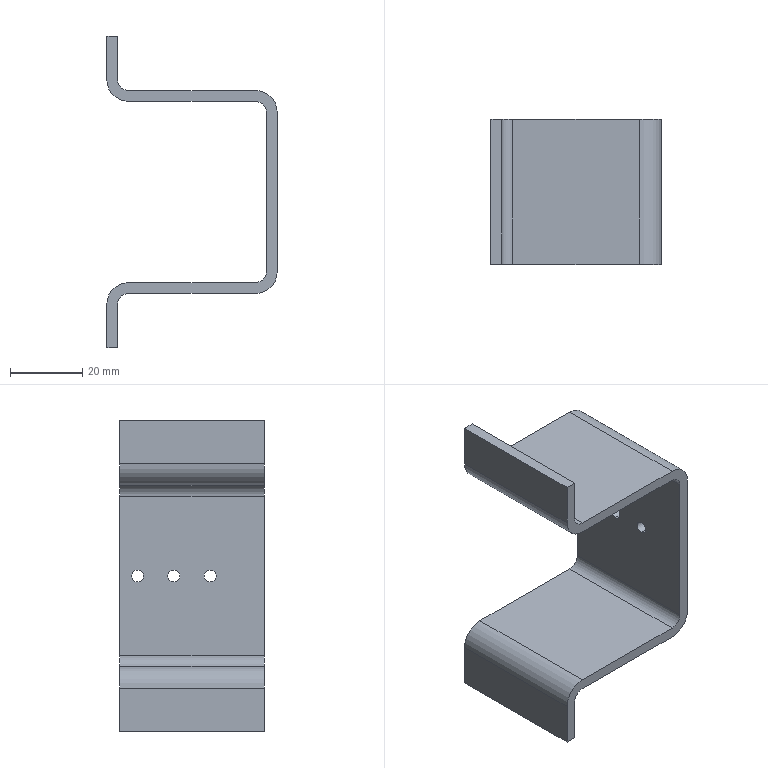Part | SolidWorks | features Fillet 2, Extrusion 1, HoleWzd 1, MoveFace 1 | 1 solid | 28 faces | box 47 x 40 x 86 mm | volume 19876 mm3 | cylinder 14 | plane 14 | commonest cylinder face diameters 3.3 x6 6 x4 12 x4
STEP:
#1=CARTESIAN_POINT('',(-1.5,35.,1.65));
#2=VERTEX_POINT('',#1);
#3=CARTESIAN_POINT('',(-1.5,35.,-1.65));
#4=VERTEX_POINT('',#3);
#5=CARTESIAN_POINT('',(-1.5,35.,0.));
#6=DIRECTION('',(1.,0.,0.));
#7=DIRECTION('',(0.,0.,-1.));
#8=AXIS2_PLACEMENT_3D('',#5,#6,#7);
#9=CIRCLE('',#8,1.65);
#10=EDGE_CURVE('',#2,#4,#9,.T.);
#11=ORIENTED_EDGE('',*,*,#10,.F.);
#12=CARTESIAN_POINT('',(1.5,35.,1.65));
#13=VERTEX_POINT('',#12);
#14=CARTESIAN_POINT('',(1.5,35.,1.65));
#15=DIRECTION('',(1.,0.,0.));
#16=VECTOR('',#15,1000.);
#17=LINE('',#14,#16);
#18=EDGE_CURVE('',#2,#13,#17,.T.);
#19=ORIENTED_EDGE('',*,*,#18,.T.);
#20=CARTESIAN_POINT('',(1.5,35.,-1.65));
#21=VERTEX_POINT('',#20);
#22=CARTESIAN_POINT('',(1.5,35.,0.));
#23=DIRECTION('',(1.,0.,0.));
#24=DIRECTION('',(0.,0.,-1.));
#25=AXIS2_PLACEMENT_3D('',#22,#23,#24);
#26=CIRCLE('',#25,1.65);
#27=EDGE_CURVE('',#13,#21,#26,.T.);
#28=ORIENTED_EDGE('',*,*,#27,.T.);
#29=CARTESIAN_POINT('',(1.5,35.,-1.65));
#30=DIRECTION('',(1.,0.,0.));
#31=VECTOR('',#30,1000.);
#32=LINE('',#29,#31);
#33=EDGE_CURVE('',#4,#21,#32,.T.);
#34=ORIENTED_EDGE('',*,*,#33,.F.);
#35=EDGE_LOOP('',(#11,#19,#28,#34));
#36=FACE_OUTER_BOUND('',#35,.T.);
#37=CARTESIAN_POINT('',(1.5,35.,0.));
#38=DIRECTION('',(1.,0.,0.));
#39=DIRECTION('',(0.,0.,-1.));
#40=AXIS2_PLACEMENT_3D('',#37,#38,#39);
#41=CYLINDRICAL_SURFACE('',#40,1.65);
#42=ADVANCED_FACE('',(#36),#41,.F.);
#43=CARTESIAN_POINT('',(-1.5,25.,1.65));
#44=VERTEX_POINT('',#43);
#45=CARTESIAN_POINT('',(-1.5,25.,-1.65));
#46=VERTEX_POINT('',#45);
#47=CARTESIAN_POINT('',(-1.5,25.,0.));
#48=DIRECTION('',(1.,0.,0.));
#49=DIRECTION('',(0.,0.,-1.));
#50=AXIS2_PLACEMENT_3D('',#47,#48,#49);
#51=CIRCLE('',#50,1.65);
#52=EDGE_CURVE('',#44,#46,#51,.T.);
#53=ORIENTED_EDGE('',*,*,#52,.F.);
#54=CARTESIAN_POINT('',(1.5,25.,1.65));
#55=VERTEX_POINT('',#54);
#56=CARTESIAN_POINT('',(1.5,25.,1.65));
#57=DIRECTION('',(1.,0.,0.));
#58=VECTOR('',#57,1000.);
#59=LINE('',#56,#58);
#60=EDGE_CURVE('',#44,#55,#59,.T.);
#61=ORIENTED_EDGE('',*,*,#60,.T.);
#62=CARTESIAN_POINT('',(1.5,25.,-1.65));
#63=VERTEX_POINT('',#62);
#64=CARTESIAN_POINT('',(1.5,25.,0.));
#65=DIRECTION('',(1.,0.,0.));
#66=DIRECTION('',(0.,0.,-1.));
#67=AXIS2_PLACEMENT_3D('',#64,#65,#66);
#68=CIRCLE('',#67,1.65);
#69=EDGE_CURVE('',#55,#63,#68,.T.);
#70=ORIENTED_EDGE('',*,*,#69,.T.);
#71=CARTESIAN_POINT('',(1.5,25.,-1.65));
#72=DIRECTION('',(1.,0.,0.));
#73=VECTOR('',#72,1000.);
#74=LINE('',#71,#73);
#75=EDGE_CURVE('',#46,#63,#74,.T.);
#76=ORIENTED_EDGE('',*,*,#75,.F.);
#77=EDGE_LOOP('',(#53,#61,#70,#76));
#78=FACE_OUTER_BOUND('',#77,.T.);
#79=CARTESIAN_POINT('',(1.5,25.,0.));
#80=DIRECTION('',(1.,0.,0.));
#81=DIRECTION('',(0.,0.,-1.));
#82=AXIS2_PLACEMENT_3D('',#79,#80,#81);
#83=CYLINDRICAL_SURFACE('',#82,1.65);
#84=ADVANCED_FACE('',(#78),#83,.F.);
#85=CARTESIAN_POINT('',(-1.5,15.,1.65));
#86=VERTEX_POINT('',#85);
#87=CARTESIAN_POINT('',(-1.5,15.,-1.65));
#88=VERTEX_POINT('',#87);
#89=CARTESIAN_POINT('',(-1.5,15.,0.));
#90=DIRECTION('',(1.,0.,0.));
#91=DIRECTION('',(0.,0.,-1.));
#92=AXIS2_PLACEMENT_3D('',#89,#90,#91);
#93=CIRCLE('',#92,1.65);
#94=EDGE_CURVE('',#86,#88,#93,.T.);
#95=ORIENTED_EDGE('',*,*,#94,.F.);
#96=CARTESIAN_POINT('',(1.5,15.,1.65));
#97=VERTEX_POINT('',#96);
#98=CARTESIAN_POINT('',(1.5,15.,1.65));
#99=DIRECTION('',(1.,0.,0.));
#100=VECTOR('',#99,1000.);
#101=LINE('',#98,#100);
#102=EDGE_CURVE('',#86,#97,#101,.T.);
#103=ORIENTED_EDGE('',*,*,#102,.T.);
#104=CARTESIAN_POINT('',(1.5,15.,-1.65));
#105=VERTEX_POINT('',#104);
#106=CARTESIAN_POINT('',(1.5,15.,0.));
#107=DIRECTION('',(1.,0.,0.));
#108=DIRECTION('',(0.,0.,-1.));
#109=AXIS2_PLACEMENT_3D('',#106,#107,#108);
#110=CIRCLE('',#109,1.65);
#111=EDGE_CURVE('',#97,#105,#110,.T.);
#112=ORIENTED_EDGE('',*,*,#111,.T.);
#113=CARTESIAN_POINT('',(1.5,15.,-1.65));
#114=DIRECTION('',(1.,0.,0.));
#115=VECTOR('',#114,1000.);
#116=LINE('',#113,#115);
#117=EDGE_CURVE('',#88,#105,#116,.T.);
#118=ORIENTED_EDGE('',*,*,#117,.F.);
#119=EDGE_LOOP('',(#95,#103,#112,#118));
#120=FACE_OUTER_BOUND('',#119,.T.);
#121=CARTESIAN_POINT('',(1.5,15.,0.));
#122=DIRECTION('',(1.,0.,0.));
#123=DIRECTION('',(0.,0.,-1.));
#124=AXIS2_PLACEMENT_3D('',#121,#122,#123);
#125=CYLINDRICAL_SURFACE('',#124,1.65);
#126=ADVANCED_FACE('',(#120),#125,.F.);
#127=CARTESIAN_POINT('',(-4.5,40.,-28.));
#128=VERTEX_POINT('',#127);
#129=CARTESIAN_POINT('',(-39.5,40.,-28.));
#130=VERTEX_POINT('',#129);
#131=CARTESIAN_POINT('',(1.5,40.,-28.));
#132=DIRECTION('',(-1.,0.,0.));
#133=VECTOR('',#132,1000.);
#134=LINE('',#131,#133);
#135=EDGE_CURVE('',#128,#130,#134,.T.);
#136=ORIENTED_EDGE('',*,*,#135,.F.);
#137=CARTESIAN_POINT('',(-4.5,0.,-28.));
#138=VERTEX_POINT('',#137);
#139=CARTESIAN_POINT('',(-4.5,40.,-28.));
#140=DIRECTION('',(0.,-1.,0.));
#141=VECTOR('',#140,1000.);
#142=LINE('',#139,#141);
#143=EDGE_CURVE('',#128,#138,#142,.T.);
#144=ORIENTED_EDGE('',*,*,#143,.T.);
#145=CARTESIAN_POINT('',(-39.5,0.,-28.));
#146=VERTEX_POINT('',#145);
#147=CARTESIAN_POINT('',(1.5,0.,-28.));
#148=DIRECTION('',(-1.,0.,0.));
#149=VECTOR('',#148,1000.);
#150=LINE('',#147,#149);
#151=EDGE_CURVE('',#138,#146,#150,.T.);
#152=ORIENTED_EDGE('',*,*,#151,.T.);
#153=CARTESIAN_POINT('',(-39.5,40.,-28.));
#154=DIRECTION('',(0.,1.,0.));
#155=VECTOR('',#154,1000.);
#156=LINE('',#153,#155);
#157=EDGE_CURVE('',#146,#130,#156,.T.);
#158=ORIENTED_EDGE('',*,*,#157,.T.);
#159=EDGE_LOOP('',(#136,#144,#152,#158));
#160=FACE_OUTER_BOUND('',#159,.T.);
#161=CARTESIAN_POINT('',(1.5,40.,-28.));
#162=DIRECTION('',(0.,0.,1.));
#163=DIRECTION('',(1.,0.,0.));
#164=AXIS2_PLACEMENT_3D('',#161,#162,#163);
#165=PLANE('',#164);
#166=ADVANCED_FACE('',(#160),#165,.F.);
#167=CARTESIAN_POINT('',(-42.5,40.,-31.));
#168=VERTEX_POINT('',#167);
#169=CARTESIAN_POINT('',(-42.5,40.,-43.));
#170=VERTEX_POINT('',#169);
#171=CARTESIAN_POINT('',(-42.5,40.,-28.));
#172=DIRECTION('',(0.,0.,-1.));
#173=VECTOR('',#172,1000.);
#174=LINE('',#171,#173);
#175=EDGE_CURVE('',#168,#170,#174,.T.);
#176=ORIENTED_EDGE('',*,*,#175,.F.);
#177=CARTESIAN_POINT('',(-42.5,0.,-31.));
#178=VERTEX_POINT('',#177);
#179=CARTESIAN_POINT('',(-42.5,0.,-31.));
#180=DIRECTION('',(0.,-1.,0.));
#181=VECTOR('',#180,1000.);
#182=LINE('',#179,#181);
#183=EDGE_CURVE('',#168,#178,#182,.T.);
#184=ORIENTED_EDGE('',*,*,#183,.T.);
#185=CARTESIAN_POINT('',(-42.5,0.,-43.));
#186=VERTEX_POINT('',#185);
#187=CARTESIAN_POINT('',(-42.5,0.,-28.));
#188=DIRECTION('',(0.,0.,-1.));
#189=VECTOR('',#188,1000.);
#190=LINE('',#187,#189);
#191=EDGE_CURVE('',#178,#186,#190,.T.);
#192=ORIENTED_EDGE('',*,*,#191,.T.);
#193=CARTESIAN_POINT('',(-42.5,40.,-43.));
#194=DIRECTION('',(0.,-1.,0.));
#195=VECTOR('',#194,1000.);
#196=LINE('',#193,#195);
#197=EDGE_CURVE('',#170,#186,#196,.T.);
#198=ORIENTED_EDGE('',*,*,#197,.F.);
#199=EDGE_LOOP('',(#176,#184,#192,#198));
#200=FACE_OUTER_BOUND('',#199,.T.);
#201=CARTESIAN_POINT('',(-42.5,40.,-28.));
#202=DIRECTION('',(-1.,0.,0.));
#203=DIRECTION('',(0.,0.,1.));
#204=AXIS2_PLACEMENT_3D('',#201,#202,#203);
#205=PLANE('',#204);
#206=ADVANCED_FACE('',(#200),#205,.F.);
#207=CARTESIAN_POINT('',(-45.5,0.,-43.));
#208=VERTEX_POINT('',#207);
#209=CARTESIAN_POINT('',(-30.5,0.,-43.));
#210=DIRECTION('',(-1.,0.,0.));
#211=VECTOR('',#210,1000.);
#212=LINE('',#209,#211);
#213=EDGE_CURVE('',#186,#208,#212,.T.);
#214=ORIENTED_EDGE('',*,*,#213,.T.);
#215=CARTESIAN_POINT('',(-45.5,40.,-43.));
#216=VERTEX_POINT('',#215);
#217=CARTESIAN_POINT('',(-45.5,40.,-43.));
#218=DIRECTION('',(0.,-1.,0.));
#219=VECTOR('',#218,1000.);
#220=LINE('',#217,#219);
#221=EDGE_CURVE('',#216,#208,#220,.T.);
#222=ORIENTED_EDGE('',*,*,#221,.F.);
#223=CARTESIAN_POINT('',(-30.5,40.,-43.));
#224=DIRECTION('',(-1.,0.,0.));
#225=VECTOR('',#224,1000.);
#226=LINE('',#223,#225);
#227=EDGE_CURVE('',#170,#216,#226,.T.);
#228=ORIENTED_EDGE('',*,*,#227,.F.);
#229=ORIENTED_EDGE('',*,*,#197,.T.);
#230=EDGE_LOOP('',(#214,#222,#228,#229));
#231=FACE_OUTER_BOUND('',#230,.T.);
#232=CARTESIAN_POINT('',(-30.5,40.,-43.));
#233=DIRECTION('',(0.,0.,1.));
#234=DIRECTION('',(1.,0.,0.));
#235=AXIS2_PLACEMENT_3D('',#232,#233,#234);
#236=PLANE('',#235);
#237=ADVANCED_FACE('',(#231),#236,.F.);
#238=CARTESIAN_POINT('',(-45.5,0.,-31.));
#239=VERTEX_POINT('',#238);
#240=CARTESIAN_POINT('',(-45.5,0.,-25.));
#241=DIRECTION('',(0.,0.,1.));
#242=VECTOR('',#241,1000.);
#243=LINE('',#240,#242);
#244=EDGE_CURVE('',#208,#239,#243,.T.);
#245=ORIENTED_EDGE('',*,*,#244,.T.);
#246=CARTESIAN_POINT('',(-45.5,40.,-31.));
#247=VERTEX_POINT('',#246);
#248=CARTESIAN_POINT('',(-45.5,40.,-31.));
#249=DIRECTION('',(0.,1.,0.));
#250=VECTOR('',#249,1000.);
#251=LINE('',#248,#250);
#252=EDGE_CURVE('',#239,#247,#251,.T.);
#253=ORIENTED_EDGE('',*,*,#252,.T.);
#254=CARTESIAN_POINT('',(-45.5,40.,-28.));
#255=DIRECTION('',(0.,0.,1.));
#256=VECTOR('',#255,1000.);
#257=LINE('',#254,#256);
#258=EDGE_CURVE('',#216,#247,#257,.T.);
#259=ORIENTED_EDGE('',*,*,#258,.F.);
#260=ORIENTED_EDGE('',*,*,#221,.T.);
#261=EDGE_LOOP('',(#245,#253,#259,#260));
#262=FACE_OUTER_BOUND('',#261,.T.);
#263=CARTESIAN_POINT('',(-45.5,40.,-25.));
#264=DIRECTION('',(1.,0.,0.));
#265=DIRECTION('',(0.,0.,-1.));
#266=AXIS2_PLACEMENT_3D('',#263,#264,#265);
#267=PLANE('',#266);
#268=ADVANCED_FACE('',(#262),#267,.F.);
#269=CARTESIAN_POINT('',(-39.5,40.,-25.));
#270=VERTEX_POINT('',#269);
#271=CARTESIAN_POINT('',(-4.5,40.,-25.));
#272=VERTEX_POINT('',#271);
#273=CARTESIAN_POINT('',(-1.5,40.,-25.));
#274=DIRECTION('',(1.,0.,0.));
#275=VECTOR('',#274,1000.);
#276=LINE('',#273,#275);
#277=EDGE_CURVE('',#270,#272,#276,.T.);
#278=ORIENTED_EDGE('',*,*,#277,.F.);
#279=CARTESIAN_POINT('',(-39.5,0.,-25.));
#280=VERTEX_POINT('',#279);
#281=CARTESIAN_POINT('',(-39.5,40.,-25.));
#282=DIRECTION('',(0.,-1.,0.));
#283=VECTOR('',#282,1000.);
#284=LINE('',#281,#283);
#285=EDGE_CURVE('',#270,#280,#284,.T.);
#286=ORIENTED_EDGE('',*,*,#285,.T.);
#287=CARTESIAN_POINT('',(-4.5,0.,-25.));
#288=VERTEX_POINT('',#287);
#289=CARTESIAN_POINT('',(-1.5,0.,-25.));
#290=DIRECTION('',(1.,0.,0.));
#291=VECTOR('',#290,1000.);
#292=LINE('',#289,#291);
#293=EDGE_CURVE('',#280,#288,#292,.T.);
#294=ORIENTED_EDGE('',*,*,#293,.T.);
#295=CARTESIAN_POINT('',(-4.5,40.,-25.));
#296=DIRECTION('',(0.,1.,0.));
#297=VECTOR('',#296,1000.);
#298=LINE('',#295,#297);
#299=EDGE_CURVE('',#288,#272,#298,.T.);
#300=ORIENTED_EDGE('',*,*,#299,.T.);
#301=EDGE_LOOP('',(#278,#286,#294,#300));
#302=FACE_OUTER_BOUND('',#301,.T.);
#303=CARTESIAN_POINT('',(-1.5,40.,-25.));
#304=DIRECTION('',(0.,0.,-1.));
#305=DIRECTION('',(-1.,0.,0.));
#306=AXIS2_PLACEMENT_3D('',#303,#304,#305);
#307=PLANE('',#306);
#308=ADVANCED_FACE('',(#302),#307,.F.);
#309=CARTESIAN_POINT('',(-1.5,35.,0.));
#310=DIRECTION('',(1.,0.,0.));
#311=DIRECTION('',(0.,0.,-1.));
#312=AXIS2_PLACEMENT_3D('',#309,#310,#311);
#313=CIRCLE('',#312,1.65);
#314=EDGE_CURVE('',#4,#2,#313,.T.);
#315=ORIENTED_EDGE('',*,*,#314,.T.);
#316=ORIENTED_EDGE('',*,*,#10,.T.);
#317=EDGE_LOOP('',(#315,#316));
#318=FACE_BOUND('',#317,.T.);
#319=CARTESIAN_POINT('',(-1.5,25.,0.));
#320=DIRECTION('',(1.,0.,0.));
#321=DIRECTION('',(0.,0.,-1.));
#322=AXIS2_PLACEMENT_3D('',#319,#320,#321);
#323=CIRCLE('',#322,1.65);
#324=EDGE_CURVE('',#46,#44,#323,.T.);
#325=ORIENTED_EDGE('',*,*,#324,.T.);
#326=ORIENTED_EDGE('',*,*,#52,.T.);
#327=EDGE_LOOP('',(#325,#326));
#328=FACE_BOUND('',#327,.T.);
#329=CARTESIAN_POINT('',(-1.5,15.,0.));
#330=DIRECTION('',(1.,0.,0.));
#331=DIRECTION('',(0.,0.,-1.));
#332=AXIS2_PLACEMENT_3D('',#329,#330,#331);
#333=CIRCLE('',#332,1.65);
#334=EDGE_CURVE('',#88,#86,#333,.T.);
#335=ORIENTED_EDGE('',*,*,#334,.T.);
#336=ORIENTED_EDGE('',*,*,#94,.T.);
#337=EDGE_LOOP('',(#335,#336));
#338=FACE_BOUND('',#337,.T.);
#339=CARTESIAN_POINT('',(-1.5,0.,-22.));
#340=VERTEX_POINT('',#339);
#341=CARTESIAN_POINT('',(-1.5,0.,22.));
#342=VERTEX_POINT('',#341);
#343=CARTESIAN_POINT('',(-1.5,0.,25.));
#344=DIRECTION('',(0.,0.,1.));
#345=VECTOR('',#344,1000.);
#346=LINE('',#343,#345);
#347=EDGE_CURVE('',#340,#342,#346,.T.);
#348=ORIENTED_EDGE('',*,*,#347,.T.);
#349=CARTESIAN_POINT('',(-1.5,40.,22.));
#350=VERTEX_POINT('',#349);
#351=CARTESIAN_POINT('',(-1.5,40.,22.));
#352=DIRECTION('',(0.,1.,0.));
#353=VECTOR('',#352,1000.);
#354=LINE('',#351,#353);
#355=EDGE_CURVE('',#342,#350,#354,.T.);
#356=ORIENTED_EDGE('',*,*,#355,.T.);
#357=CARTESIAN_POINT('',(-1.5,40.,-22.));
#358=VERTEX_POINT('',#357);
#359=CARTESIAN_POINT('',(-1.5,40.,25.));
#360=DIRECTION('',(0.,0.,1.));
#361=VECTOR('',#360,1000.);
#362=LINE('',#359,#361);
#363=EDGE_CURVE('',#358,#350,#362,.T.);
#364=ORIENTED_EDGE('',*,*,#363,.F.);
#365=CARTESIAN_POINT('',(-1.5,0.,-22.));
#366=DIRECTION('',(0.,-1.,0.));
#367=VECTOR('',#366,1000.);
#368=LINE('',#365,#367);
#369=EDGE_CURVE('',#358,#340,#368,.T.);
#370=ORIENTED_EDGE('',*,*,#369,.T.);
#371=EDGE_LOOP('',(#348,#356,#364,#370));
#372=FACE_OUTER_BOUND('',#371,.T.);
#373=CARTESIAN_POINT('',(-1.5,40.,25.));
#374=DIRECTION('',(1.,0.,0.));
#375=DIRECTION('',(0.,0.,-1.));
#376=AXIS2_PLACEMENT_3D('',#373,#374,#375);
#377=PLANE('',#376);
#378=ADVANCED_FACE('',(#318,#328,#338,#372),#377,.F.);
#379=CARTESIAN_POINT('',(-4.5,0.,25.));
#380=VERTEX_POINT('',#379);
#381=CARTESIAN_POINT('',(-39.5,0.,25.));
#382=VERTEX_POINT('',#381);
#383=CARTESIAN_POINT('',(-1.5,0.,25.));
#384=DIRECTION('',(-1.,0.,0.));
#385=VECTOR('',#384,1000.);
#386=LINE('',#383,#385);
#387=EDGE_CURVE('',#380,#382,#386,.T.);
#388=ORIENTED_EDGE('',*,*,#387,.T.);
#389=CARTESIAN_POINT('',(-39.5,40.,25.));
#390=VERTEX_POINT('',#389);
#391=CARTESIAN_POINT('',(-39.5,40.,25.));
#392=DIRECTION('',(0.,1.,0.));
#393=VECTOR('',#392,1000.);
#394=LINE('',#391,#393);
#395=EDGE_CURVE('',#382,#390,#394,.T.);
#396=ORIENTED_EDGE('',*,*,#395,.T.);
#397=CARTESIAN_POINT('',(-4.5,40.,25.));
#398=VERTEX_POINT('',#397);
#399=CARTESIAN_POINT('',(-1.5,40.,25.));
#400=DIRECTION('',(-1.,0.,0.));
#401=VECTOR('',#400,1000.);
#402=LINE('',#399,#401);
#403=EDGE_CURVE('',#398,#390,#402,.T.);
#404=ORIENTED_EDGE('',*,*,#403,.F.);
#405=CARTESIAN_POINT('',(-4.5,0.,25.));
#406=DIRECTION('',(0.,-1.,0.));
#407=VECTOR('',#406,1000.);
#408=LINE('',#405,#407);
#409=EDGE_CURVE('',#398,#380,#408,.T.);
#410=ORIENTED_EDGE('',*,*,#409,.T.);
#411=EDGE_LOOP('',(#388,#396,#404,#410));
#412=FACE_OUTER_BOUND('',#411,.T.);
#413=CARTESIAN_POINT('',(-1.5,40.,25.));
#414=DIRECTION('',(0.,0.,1.));
#415=DIRECTION('',(1.,0.,0.));
#416=AXIS2_PLACEMENT_3D('',#413,#414,#415);
#417=PLANE('',#416);
#418=ADVANCED_FACE('',(#412),#417,.F.);
#419=CARTESIAN_POINT('',(-45.5,40.,31.));
#420=VERTEX_POINT('',#419);
#421=CARTESIAN_POINT('',(-45.5,40.,43.));
#422=VERTEX_POINT('',#421);
#423=CARTESIAN_POINT('',(-45.5,40.,25.));
#424=DIRECTION('',(0.,0.,1.));
#425=VECTOR('',#424,1000.);
#426=LINE('',#423,#425);
#427=EDGE_CURVE('',#420,#422,#426,.T.);
#428=ORIENTED_EDGE('',*,*,#427,.F.);
#429=CARTESIAN_POINT('',(-45.5,0.,31.));
#430=VERTEX_POINT('',#429);
#431=CARTESIAN_POINT('',(-45.5,40.,31.));
#432=DIRECTION('',(0.,-1.,0.));
#433=VECTOR('',#432,1000.);
#434=LINE('',#431,#433);
#435=EDGE_CURVE('',#420,#430,#434,.T.);
#436=ORIENTED_EDGE('',*,*,#435,.T.);
#437=CARTESIAN_POINT('',(-45.5,0.,43.));
#438=VERTEX_POINT('',#437);
#439=CARTESIAN_POINT('',(-45.5,0.,28.));
#440=DIRECTION('',(0.,0.,1.));
#441=VECTOR('',#440,1000.);
#442=LINE('',#439,#441);
#443=EDGE_CURVE('',#430,#438,#442,.T.);
#444=ORIENTED_EDGE('',*,*,#443,.T.);
#445=CARTESIAN_POINT('',(-45.5,40.,43.));
#446=DIRECTION('',(0.,-1.,0.));
#447=VECTOR('',#446,1000.);
#448=LINE('',#445,#447);
#449=EDGE_CURVE('',#422,#438,#448,.T.);
#450=ORIENTED_EDGE('',*,*,#449,.F.);
#451=EDGE_LOOP('',(#428,#436,#444,#450));
#452=FACE_OUTER_BOUND('',#451,.T.);
#453=CARTESIAN_POINT('',(-45.5,40.,28.));
#454=DIRECTION('',(1.,0.,0.));
#455=DIRECTION('',(0.,0.,-1.));
#456=AXIS2_PLACEMENT_3D('',#453,#454,#455);
#457=PLANE('',#456);
#458=ADVANCED_FACE('',(#452),#457,.F.);
#459=CARTESIAN_POINT('',(-42.5,0.,43.));
#460=VERTEX_POINT('',#459);
#461=CARTESIAN_POINT('',(-30.5,0.,43.));
#462=DIRECTION('',(1.,0.,0.));
#463=VECTOR('',#462,1000.);
#464=LINE('',#461,#463);
#465=EDGE_CURVE('',#438,#460,#464,.T.);
#466=ORIENTED_EDGE('',*,*,#465,.T.);
#467=CARTESIAN_POINT('',(-42.5,40.,43.));
#468=VERTEX_POINT('',#467);
#469=CARTESIAN_POINT('',(-42.5,40.,43.));
#470=DIRECTION('',(0.,-1.,0.));
#471=VECTOR('',#470,1000.);
#472=LINE('',#469,#471);
#473=EDGE_CURVE('',#468,#460,#472,.T.);
#474=ORIENTED_EDGE('',*,*,#473,.F.);
#475=CARTESIAN_POINT('',(-30.5,40.,43.));
#476=DIRECTION('',(1.,0.,0.));
#477=VECTOR('',#476,1000.);
#478=LINE('',#475,#477);
#479=EDGE_CURVE('',#422,#468,#478,.T.);
#480=ORIENTED_EDGE('',*,*,#479,.F.);
#481=ORIENTED_EDGE('',*,*,#449,.T.);
#482=EDGE_LOOP('',(#466,#474,#480,#481));
#483=FACE_OUTER_BOUND('',#482,.T.);
#484=CARTESIAN_POINT('',(-30.5,40.,43.));
#485=DIRECTION('',(0.,0.,-1.));
#486=DIRECTION('',(-1.,0.,0.));
#487=AXIS2_PLACEMENT_3D('',#484,#485,#486);
#488=PLANE('',#487);
#489=ADVANCED_FACE('',(#483),#488,.F.);
#490=CARTESIAN_POINT('',(-42.5,0.,31.));
#491=VERTEX_POINT('',#490);
#492=CARTESIAN_POINT('',(-42.5,0.,28.));
#493=DIRECTION('',(0.,0.,-1.));
#494=VECTOR('',#493,1000.);
#495=LINE('',#492,#494);
#496=EDGE_CURVE('',#460,#491,#495,.T.);
#497=ORIENTED_EDGE('',*,*,#496,.T.);
#498=CARTESIAN_POINT('',(-42.5,40.,31.));
#499=VERTEX_POINT('',#498);
#500=CARTESIAN_POINT('',(-42.5,40.,31.));
#501=DIRECTION('',(0.,1.,0.));
#502=VECTOR('',#501,1000.);
#503=LINE('',#500,#502);
#504=EDGE_CURVE('',#491,#499,#503,.T.);
#505=ORIENTED_EDGE('',*,*,#504,.T.);
#506=CARTESIAN_POINT('',(-42.5,40.,28.));
#507=DIRECTION('',(0.,0.,-1.));
#508=VECTOR('',#507,1000.);
#509=LINE('',#506,#508);
#510=EDGE_CURVE('',#468,#499,#509,.T.);
#511=ORIENTED_EDGE('',*,*,#510,.F.);
#512=ORIENTED_EDGE('',*,*,#473,.T.);
#513=EDGE_LOOP('',(#497,#505,#511,#512));
#514=FACE_OUTER_BOUND('',#513,.T.);
#515=CARTESIAN_POINT('',(-42.5,40.,28.));
#516=DIRECTION('',(-1.,0.,0.));
#517=DIRECTION('',(0.,0.,1.));
#518=AXIS2_PLACEMENT_3D('',#515,#516,#517);
#519=PLANE('',#518);
#520=ADVANCED_FACE('',(#514),#519,.F.);
#521=CARTESIAN_POINT('',(-39.5,0.,28.));
#522=VERTEX_POINT('',#521);
#523=CARTESIAN_POINT('',(-4.5,0.,28.));
#524=VERTEX_POINT('',#523);
#525=CARTESIAN_POINT('',(1.5,0.,28.));
#526=DIRECTION('',(1.,0.,0.));
#527=VECTOR('',#526,1000.);
#528=LINE('',#525,#527);
#529=EDGE_CURVE('',#522,#524,#528,.T.);
#530=ORIENTED_EDGE('',*,*,#529,.T.);
#531=CARTESIAN_POINT('',(-4.5,40.,28.));
#532=VERTEX_POINT('',#531);
#533=CARTESIAN_POINT('',(-4.5,40.,28.));
#534=DIRECTION('',(0.,1.,0.));
#535=VECTOR('',#534,1000.);
#536=LINE('',#533,#535);
#537=EDGE_CURVE('',#524,#532,#536,.T.);
#538=ORIENTED_EDGE('',*,*,#537,.T.);
#539=CARTESIAN_POINT('',(-39.5,40.,28.));
#540=VERTEX_POINT('',#539);
#541=CARTESIAN_POINT('',(1.5,40.,28.));
#542=DIRECTION('',(1.,0.,0.));
#543=VECTOR('',#542,1000.);
#544=LINE('',#541,#543);
#545=EDGE_CURVE('',#540,#532,#544,.T.);
#546=ORIENTED_EDGE('',*,*,#545,.F.);
#547=CARTESIAN_POINT('',(-39.5,0.,28.));
#548=DIRECTION('',(0.,-1.,0.));
#549=VECTOR('',#548,1000.);
#550=LINE('',#547,#549);
#551=EDGE_CURVE('',#540,#522,#550,.T.);
#552=ORIENTED_EDGE('',*,*,#551,.T.);
#553=EDGE_LOOP('',(#530,#538,#546,#552));
#554=FACE_OUTER_BOUND('',#553,.T.);
#555=CARTESIAN_POINT('',(1.5,40.,28.));
#556=DIRECTION('',(0.,0.,-1.));
#557=DIRECTION('',(-1.,0.,0.));
#558=AXIS2_PLACEMENT_3D('',#555,#556,#557);
#559=PLANE('',#558);
#560=ADVANCED_FACE('',(#554),#559,.F.);
#561=CARTESIAN_POINT('',(1.5,35.,0.));
#562=DIRECTION('',(1.,0.,0.));
#563=DIRECTION('',(0.,0.,-1.));
#564=AXIS2_PLACEMENT_3D('',#561,#562,#563);
#565=CIRCLE('',#564,1.65);
#566=EDGE_CURVE('',#21,#13,#565,.T.);
#567=ORIENTED_EDGE('',*,*,#566,.F.);
#568=ORIENTED_EDGE('',*,*,#27,.F.);
#569=EDGE_LOOP('',(#567,#568));
#570=FACE_BOUND('',#569,.T.);
#571=CARTESIAN_POINT('',(1.5,25.,0.));
#572=DIRECTION('',(1.,0.,0.));
#573=DIRECTION('',(0.,0.,-1.));
#574=AXIS2_PLACEMENT_3D('',#571,#572,#573);
#575=CIRCLE('',#574,1.65);
#576=EDGE_CURVE('',#63,#55,#575,.T.);
#577=ORIENTED_EDGE('',*,*,#576,.F.);
#578=ORIENTED_EDGE('',*,*,#69,.F.);
#579=EDGE_LOOP('',(#577,#578));
#580=FACE_BOUND('',#579,.T.);
#581=CARTESIAN_POINT('',(1.5,15.,0.));
#582=DIRECTION('',(1.,0.,0.));
#583=DIRECTION('',(0.,0.,-1.));
#584=AXIS2_PLACEMENT_3D('',#581,#582,#583);
#585=CIRCLE('',#584,1.65);
#586=EDGE_CURVE('',#105,#97,#585,.T.);
#587=ORIENTED_EDGE('',*,*,#586,.F.);
#588=ORIENTED_EDGE('',*,*,#111,.F.);
#589=EDGE_LOOP('',(#587,#588));
#590=FACE_BOUND('',#589,.T.);
#591=CARTESIAN_POINT('',(1.5,40.,22.));
#592=VERTEX_POINT('',#591);
#593=CARTESIAN_POINT('',(1.5,40.,-22.));
#594=VERTEX_POINT('',#593);
#595=CARTESIAN_POINT('',(1.5,40.,-25.));
#596=DIRECTION('',(0.,0.,-1.));
#597=VECTOR('',#596,1000.);
#598=LINE('',#595,#597);
#599=EDGE_CURVE('',#592,#594,#598,.T.);
#600=ORIENTED_EDGE('',*,*,#599,.F.);
#601=CARTESIAN_POINT('',(1.5,0.,22.));
#602=VERTEX_POINT('',#601);
#603=CARTESIAN_POINT('',(1.5,40.,22.));
#604=DIRECTION('',(0.,-1.,0.));
#605=VECTOR('',#604,1000.);
#606=LINE('',#603,#605);
#607=EDGE_CURVE('',#592,#602,#606,.T.);
#608=ORIENTED_EDGE('',*,*,#607,.T.);
#609=CARTESIAN_POINT('',(1.5,0.,-22.));
#610=VERTEX_POINT('',#609);
#611=CARTESIAN_POINT('',(1.5,0.,25.));
#612=DIRECTION('',(0.,0.,-1.));
#613=VECTOR('',#612,1000.);
#614=LINE('',#611,#613);
#615=EDGE_CURVE('',#602,#610,#614,.T.);
#616=ORIENTED_EDGE('',*,*,#615,.T.);
#617=CARTESIAN_POINT('',(1.5,40.,-22.));
#618=DIRECTION('',(0.,1.,0.));
#619=VECTOR('',#618,1000.);
#620=LINE('',#617,#619);
#621=EDGE_CURVE('',#610,#594,#620,.T.);
#622=ORIENTED_EDGE('',*,*,#621,.T.);
#623=EDGE_LOOP('',(#600,#608,#616,#622));
#624=FACE_OUTER_BOUND('',#623,.T.);
#625=CARTESIAN_POINT('',(1.5,40.,25.));
#626=DIRECTION('',(-1.,0.,0.));
#627=DIRECTION('',(0.,0.,1.));
#628=AXIS2_PLACEMENT_3D('',#625,#626,#627);
#629=PLANE('',#628);
#630=ADVANCED_FACE('',(#570,#580,#590,#624),#629,.F.);
#631=ORIENTED_EDGE('',*,*,#403,.T.);
#632=CARTESIAN_POINT('',(-39.5,40.,31.));
#633=DIRECTION('',(0.,1.,0.));
#634=DIRECTION('',(0.,0.,1.));
#635=AXIS2_PLACEMENT_3D('',#632,#633,#634);
#636=CIRCLE('',#635,6.);
#637=EDGE_CURVE('',#390,#420,#636,.T.);
#638=ORIENTED_EDGE('',*,*,#637,.T.);
#639=ORIENTED_EDGE('',*,*,#427,.T.);
#640=ORIENTED_EDGE('',*,*,#479,.T.);
#641=ORIENTED_EDGE('',*,*,#510,.T.);
#642=CARTESIAN_POINT('',(-39.5,40.,31.));
#643=DIRECTION('',(0.,-1.,0.));
#644=DIRECTION('',(0.,0.,1.));
#645=AXIS2_PLACEMENT_3D('',#642,#643,#644);
#646=CIRCLE('',#645,3.);
#647=EDGE_CURVE('',#499,#540,#646,.T.);
#648=ORIENTED_EDGE('',*,*,#647,.T.);
#649=ORIENTED_EDGE('',*,*,#545,.T.);
#650=CARTESIAN_POINT('',(-4.5,40.,22.));
#651=DIRECTION('',(0.,1.,0.));
#652=DIRECTION('',(0.,0.,1.));
#653=AXIS2_PLACEMENT_3D('',#650,#651,#652);
#654=CIRCLE('',#653,6.);
#655=EDGE_CURVE('',#532,#592,#654,.T.);
#656=ORIENTED_EDGE('',*,*,#655,.T.);
#657=ORIENTED_EDGE('',*,*,#599,.T.);
#658=CARTESIAN_POINT('',(-4.5,40.,-22.));
#659=DIRECTION('',(0.,1.,0.));
#660=DIRECTION('',(0.,0.,1.));
#661=AXIS2_PLACEMENT_3D('',#658,#659,#660);
#662=CIRCLE('',#661,6.);
#663=EDGE_CURVE('',#594,#128,#662,.T.);
#664=ORIENTED_EDGE('',*,*,#663,.T.);
#665=ORIENTED_EDGE('',*,*,#135,.T.);
#666=CARTESIAN_POINT('',(-39.5,40.,-31.));
#667=DIRECTION('',(0.,-1.,0.));
#668=DIRECTION('',(0.,0.,1.));
#669=AXIS2_PLACEMENT_3D('',#666,#667,#668);
#670=CIRCLE('',#669,3.);
#671=EDGE_CURVE('',#130,#168,#670,.T.);
#672=ORIENTED_EDGE('',*,*,#671,.T.);
#673=ORIENTED_EDGE('',*,*,#175,.T.);
#674=ORIENTED_EDGE('',*,*,#227,.T.);
#675=ORIENTED_EDGE('',*,*,#258,.T.);
#676=CARTESIAN_POINT('',(-39.5,40.,-31.));
#677=DIRECTION('',(0.,1.,0.));
#678=DIRECTION('',(0.,0.,1.));
#679=AXIS2_PLACEMENT_3D('',#676,#677,#678);
#680=CIRCLE('',#679,6.);
#681=EDGE_CURVE('',#247,#270,#680,.T.);
#682=ORIENTED_EDGE('',*,*,#681,.T.);
#683=ORIENTED_EDGE('',*,*,#277,.T.);
#684=CARTESIAN_POINT('',(-4.5,40.,-22.));
#685=DIRECTION('',(0.,-1.,0.));
#686=DIRECTION('',(0.,0.,1.));
#687=AXIS2_PLACEMENT_3D('',#684,#685,#686);
#688=CIRCLE('',#687,3.);
#689=EDGE_CURVE('',#272,#358,#688,.T.);
#690=ORIENTED_EDGE('',*,*,#689,.T.);
#691=ORIENTED_EDGE('',*,*,#363,.T.);
#692=CARTESIAN_POINT('',(-4.5,40.,22.));
#693=DIRECTION('',(0.,-1.,0.));
#694=DIRECTION('',(0.,0.,1.));
#695=AXIS2_PLACEMENT_3D('',#692,#693,#694);
#696=CIRCLE('',#695,3.);
#697=EDGE_CURVE('',#350,#398,#696,.T.);
#698=ORIENTED_EDGE('',*,*,#697,.T.);
#699=EDGE_LOOP('',(#631,#638,#639,#640,#641,#648,#649,#656,#657,#664,#665,#672,#673,#674,#675,#682,#683,#690,#691,#698));
#700=FACE_OUTER_BOUND('',#699,.T.);
#701=CARTESIAN_POINT('',(0.,40.,0.));
#702=DIRECTION('',(0.,1.,0.));
#703=DIRECTION('',(0.,0.,1.));
#704=AXIS2_PLACEMENT_3D('',#701,#702,#703);
#705=PLANE('',#704);
#706=ADVANCED_FACE('',(#700),#705,.T.);
#707=ORIENTED_EDGE('',*,*,#443,.F.);
#708=CARTESIAN_POINT('',(-39.5,0.,31.));
#709=DIRECTION('',(0.,-1.,0.));
#710=DIRECTION('',(0.,0.,1.));
#711=AXIS2_PLACEMENT_3D('',#708,#709,#710);
#712=CIRCLE('',#711,6.);
#713=EDGE_CURVE('',#430,#382,#712,.T.);
#714=ORIENTED_EDGE('',*,*,#713,.T.);
#715=ORIENTED_EDGE('',*,*,#387,.F.);
#716=CARTESIAN_POINT('',(-4.5,0.,22.));
#717=DIRECTION('',(0.,1.,0.));
#718=DIRECTION('',(0.,0.,1.));
#719=AXIS2_PLACEMENT_3D('',#716,#717,#718);
#720=CIRCLE('',#719,3.);
#721=EDGE_CURVE('',#380,#342,#720,.T.);
#722=ORIENTED_EDGE('',*,*,#721,.T.);
#723=ORIENTED_EDGE('',*,*,#347,.F.);
#724=CARTESIAN_POINT('',(-4.5,0.,-22.));
#725=DIRECTION('',(0.,1.,0.));
#726=DIRECTION('',(0.,0.,1.));
#727=AXIS2_PLACEMENT_3D('',#724,#725,#726);
#728=CIRCLE('',#727,3.);
#729=EDGE_CURVE('',#340,#288,#728,.T.);
#730=ORIENTED_EDGE('',*,*,#729,.T.);
#731=ORIENTED_EDGE('',*,*,#293,.F.);
#732=CARTESIAN_POINT('',(-39.5,0.,-31.));
#733=DIRECTION('',(0.,-1.,0.));
#734=DIRECTION('',(0.,0.,1.));
#735=AXIS2_PLACEMENT_3D('',#732,#733,#734);
#736=CIRCLE('',#735,6.);
#737=EDGE_CURVE('',#280,#239,#736,.T.);
#738=ORIENTED_EDGE('',*,*,#737,.T.);
#739=ORIENTED_EDGE('',*,*,#244,.F.);
#740=ORIENTED_EDGE('',*,*,#213,.F.);
#741=ORIENTED_EDGE('',*,*,#191,.F.);
#742=CARTESIAN_POINT('',(-39.5,0.,-31.));
#743=DIRECTION('',(0.,1.,0.));
#744=DIRECTION('',(0.,0.,1.));
#745=AXIS2_PLACEMENT_3D('',#742,#743,#744);
#746=CIRCLE('',#745,3.);
#747=EDGE_CURVE('',#178,#146,#746,.T.);
#748=ORIENTED_EDGE('',*,*,#747,.T.);
#749=ORIENTED_EDGE('',*,*,#151,.F.);
#750=CARTESIAN_POINT('',(-4.5,0.,-22.));
#751=DIRECTION('',(0.,-1.,0.));
#752=DIRECTION('',(0.,0.,1.));
#753=AXIS2_PLACEMENT_3D('',#750,#751,#752);
#754=CIRCLE('',#753,6.);
#755=EDGE_CURVE('',#138,#610,#754,.T.);
#756=ORIENTED_EDGE('',*,*,#755,.T.);
#757=ORIENTED_EDGE('',*,*,#615,.F.);
#758=CARTESIAN_POINT('',(-4.5,0.,22.));
#759=DIRECTION('',(0.,-1.,0.));
#760=DIRECTION('',(0.,0.,1.));
#761=AXIS2_PLACEMENT_3D('',#758,#759,#760);
#762=CIRCLE('',#761,6.);
#763=EDGE_CURVE('',#602,#524,#762,.T.);
#764=ORIENTED_EDGE('',*,*,#763,.T.);
#765=ORIENTED_EDGE('',*,*,#529,.F.);
#766=CARTESIAN_POINT('',(-39.5,0.,31.));
#767=DIRECTION('',(0.,1.,0.));
#768=DIRECTION('',(0.,0.,1.));
#769=AXIS2_PLACEMENT_3D('',#766,#767,#768);
#770=CIRCLE('',#769,3.);
#771=EDGE_CURVE('',#522,#491,#770,.T.);
#772=ORIENTED_EDGE('',*,*,#771,.T.);
#773=ORIENTED_EDGE('',*,*,#496,.F.);
#774=ORIENTED_EDGE('',*,*,#465,.F.);
#775=EDGE_LOOP('',(#707,#714,#715,#722,#723,#730,#731,#738,#739,#740,#741,#748,#749,#756,#757,#764,#765,#772,#773,#774));
#776=FACE_OUTER_BOUND('',#775,.T.);
#777=CARTESIAN_POINT('',(0.,0.,0.));
#778=DIRECTION('',(0.,1.,0.));
#779=DIRECTION('',(0.,0.,1.));
#780=AXIS2_PLACEMENT_3D('',#777,#778,#779);
#781=PLANE('',#780);
#782=ADVANCED_FACE('',(#776),#781,.F.);
#783=ORIENTED_EDGE('',*,*,#647,.F.);
#784=ORIENTED_EDGE('',*,*,#504,.F.);
#785=ORIENTED_EDGE('',*,*,#771,.F.);
#786=ORIENTED_EDGE('',*,*,#551,.F.);
#787=EDGE_LOOP('',(#783,#784,#785,#786));
#788=FACE_OUTER_BOUND('',#787,.T.);
#789=CARTESIAN_POINT('',(-39.5,40.,31.));
#790=DIRECTION('',(0.,1.,0.));
#791=DIRECTION('',(0.,0.,1.));
#792=AXIS2_PLACEMENT_3D('',#789,#790,#791);
#793=CYLINDRICAL_SURFACE('',#792,3.);
#794=ADVANCED_FACE('',(#788),#793,.F.);
#795=ORIENTED_EDGE('',*,*,#697,.F.);
#796=ORIENTED_EDGE('',*,*,#355,.F.);
#797=ORIENTED_EDGE('',*,*,#721,.F.);
#798=ORIENTED_EDGE('',*,*,#409,.F.);
#799=EDGE_LOOP('',(#795,#796,#797,#798));
#800=FACE_OUTER_BOUND('',#799,.T.);
#801=CARTESIAN_POINT('',(-4.5,40.,22.));
#802=DIRECTION('',(0.,1.,0.));
#803=DIRECTION('',(0.,0.,1.));
#804=AXIS2_PLACEMENT_3D('',#801,#802,#803);
#805=CYLINDRICAL_SURFACE('',#804,3.);
#806=ADVANCED_FACE('',(#800),#805,.F.);
#807=ORIENTED_EDGE('',*,*,#689,.F.);
#808=ORIENTED_EDGE('',*,*,#299,.F.);
#809=ORIENTED_EDGE('',*,*,#729,.F.);
#810=ORIENTED_EDGE('',*,*,#369,.F.);
#811=EDGE_LOOP('',(#807,#808,#809,#810));
#812=FACE_OUTER_BOUND('',#811,.T.);
#813=CARTESIAN_POINT('',(-4.5,40.,-22.));
#814=DIRECTION('',(0.,1.,0.));
#815=DIRECTION('',(0.,0.,1.));
#816=AXIS2_PLACEMENT_3D('',#813,#814,#815);
#817=CYLINDRICAL_SURFACE('',#816,3.);
#818=ADVANCED_FACE('',(#812),#817,.F.);
#819=ORIENTED_EDGE('',*,*,#671,.F.);
#820=ORIENTED_EDGE('',*,*,#157,.F.);
#821=ORIENTED_EDGE('',*,*,#747,.F.);
#822=ORIENTED_EDGE('',*,*,#183,.F.);
#823=EDGE_LOOP('',(#819,#820,#821,#822));
#824=FACE_OUTER_BOUND('',#823,.T.);
#825=CARTESIAN_POINT('',(-39.5,40.,-31.));
#826=DIRECTION('',(0.,1.,0.));
#827=DIRECTION('',(0.,0.,1.));
#828=AXIS2_PLACEMENT_3D('',#825,#826,#827);
#829=CYLINDRICAL_SURFACE('',#828,3.);
#830=ADVANCED_FACE('',(#824),#829,.F.);
#831=ORIENTED_EDGE('',*,*,#637,.F.);
#832=ORIENTED_EDGE('',*,*,#395,.F.);
#833=ORIENTED_EDGE('',*,*,#713,.F.);
#834=ORIENTED_EDGE('',*,*,#435,.F.);
#835=EDGE_LOOP('',(#831,#832,#833,#834));
#836=FACE_OUTER_BOUND('',#835,.T.);
#837=CARTESIAN_POINT('',(-39.5,40.,31.));
#838=DIRECTION('',(0.,-1.,0.));
#839=DIRECTION('',(0.,0.,-1.));
#840=AXIS2_PLACEMENT_3D('',#837,#838,#839);
#841=CYLINDRICAL_SURFACE('',#840,6.);
#842=ADVANCED_FACE('',(#836),#841,.T.);
#843=ORIENTED_EDGE('',*,*,#655,.F.);
#844=ORIENTED_EDGE('',*,*,#537,.F.);
#845=ORIENTED_EDGE('',*,*,#763,.F.);
#846=ORIENTED_EDGE('',*,*,#607,.F.);
#847=EDGE_LOOP('',(#843,#844,#845,#846));
#848=FACE_OUTER_BOUND('',#847,.T.);
#849=CARTESIAN_POINT('',(-4.5,40.,22.));
#850=DIRECTION('',(0.,-1.,0.));
#851=DIRECTION('',(0.,0.,-1.));
#852=AXIS2_PLACEMENT_3D('',#849,#850,#851);
#853=CYLINDRICAL_SURFACE('',#852,6.);
#854=ADVANCED_FACE('',(#848),#853,.T.);
#855=ORIENTED_EDGE('',*,*,#663,.F.);
#856=ORIENTED_EDGE('',*,*,#621,.F.);
#857=ORIENTED_EDGE('',*,*,#755,.F.);
#858=ORIENTED_EDGE('',*,*,#143,.F.);
#859=EDGE_LOOP('',(#855,#856,#857,#858));
#860=FACE_OUTER_BOUND('',#859,.T.);
#861=CARTESIAN_POINT('',(-4.5,40.,-22.));
#862=DIRECTION('',(0.,-1.,0.));
#863=DIRECTION('',(0.,0.,-1.));
#864=AXIS2_PLACEMENT_3D('',#861,#862,#863);
#865=CYLINDRICAL_SURFACE('',#864,6.);
#866=ADVANCED_FACE('',(#860),#865,.T.);
#867=ORIENTED_EDGE('',*,*,#681,.F.);
#868=ORIENTED_EDGE('',*,*,#252,.F.);
#869=ORIENTED_EDGE('',*,*,#737,.F.);
#870=ORIENTED_EDGE('',*,*,#285,.F.);
#871=EDGE_LOOP('',(#867,#868,#869,#870));
#872=FACE_OUTER_BOUND('',#871,.T.);
#873=CARTESIAN_POINT('',(-39.5,40.,-31.));
#874=DIRECTION('',(0.,-1.,0.));
#875=DIRECTION('',(0.,0.,-1.));
#876=AXIS2_PLACEMENT_3D('',#873,#874,#875);
#877=CYLINDRICAL_SURFACE('',#876,6.);
#878=ADVANCED_FACE('',(#872),#877,.T.);
#879=ORIENTED_EDGE('',*,*,#102,.F.);
#880=ORIENTED_EDGE('',*,*,#334,.F.);
#881=ORIENTED_EDGE('',*,*,#117,.T.);
#882=ORIENTED_EDGE('',*,*,#586,.T.);
#883=EDGE_LOOP('',(#879,#880,#881,#882));
#884=FACE_OUTER_BOUND('',#883,.T.);
#885=CARTESIAN_POINT('',(1.5,15.,0.));
#886=DIRECTION('',(1.,0.,0.));
#887=DIRECTION('',(0.,0.,-1.));
#888=AXIS2_PLACEMENT_3D('',#885,#886,#887);
#889=CYLINDRICAL_SURFACE('',#888,1.65);
#890=ADVANCED_FACE('',(#884),#889,.F.);
#891=ORIENTED_EDGE('',*,*,#60,.F.);
#892=ORIENTED_EDGE('',*,*,#324,.F.);
#893=ORIENTED_EDGE('',*,*,#75,.T.);
#894=ORIENTED_EDGE('',*,*,#576,.T.);
#895=EDGE_LOOP('',(#891,#892,#893,#894));
#896=FACE_OUTER_BOUND('',#895,.T.);
#897=CARTESIAN_POINT('',(1.5,25.,0.));
#898=DIRECTION('',(1.,0.,0.));
#899=DIRECTION('',(0.,0.,-1.));
#900=AXIS2_PLACEMENT_3D('',#897,#898,#899);
#901=CYLINDRICAL_SURFACE('',#900,1.65);
#902=ADVANCED_FACE('',(#896),#901,.F.);
#903=ORIENTED_EDGE('',*,*,#18,.F.);
#904=ORIENTED_EDGE('',*,*,#314,.F.);
#905=ORIENTED_EDGE('',*,*,#33,.T.);
#906=ORIENTED_EDGE('',*,*,#566,.T.);
#907=EDGE_LOOP('',(#903,#904,#905,#906));
#908=FACE_OUTER_BOUND('',#907,.T.);
#909=CARTESIAN_POINT('',(1.5,35.,0.));
#910=DIRECTION('',(1.,0.,0.));
#911=DIRECTION('',(0.,0.,-1.));
#912=AXIS2_PLACEMENT_3D('',#909,#910,#911);
#913=CYLINDRICAL_SURFACE('',#912,1.65);
#914=ADVANCED_FACE('',(#908),#913,.F.);
#915=CLOSED_SHELL('',(#42,#84,#126,#166,#206,#237,#268,#308,#378,#418,#458,#489,#520,#560,#630,#706,#782,#794,#806,#818,#830,#842,#854,#866,#878,#890,#902,#914));
#916=MANIFOLD_SOLID_BREP('',#915);
#917=CARTESIAN_POINT('',(0.,0.,0.));
#918=DIRECTION('',(0.,0.,1.));
#919=DIRECTION('',(1.,0.,0.));
#920=AXIS2_PLACEMENT_3D('',#917,#918,#919);
#921=(LENGTH_UNIT()NAMED_UNIT(*)SI_UNIT(.MILLI.,.METRE.));
#922=UNCERTAINTY_MEASURE_WITH_UNIT(LENGTH_MEASURE(0.00001),#921,'','');
#923=(NAMED_UNIT(*)PLANE_ANGLE_UNIT()SI_UNIT($,.RADIAN.));
#924=(NAMED_UNIT(*)SI_UNIT($,.STERADIAN.)SOLID_ANGLE_UNIT());
#925=(GEOMETRIC_REPRESENTATION_CONTEXT(3)GLOBAL_UNCERTAINTY_ASSIGNED_CONTEXT((#922))GLOBAL_UNIT_ASSIGNED_CONTEXT((#921,#923,#924))REPRESENTATION_CONTEXT('',''));
#926=ADVANCED_BREP_SHAPE_REPRESENTATION('',(#916,#920),#925);